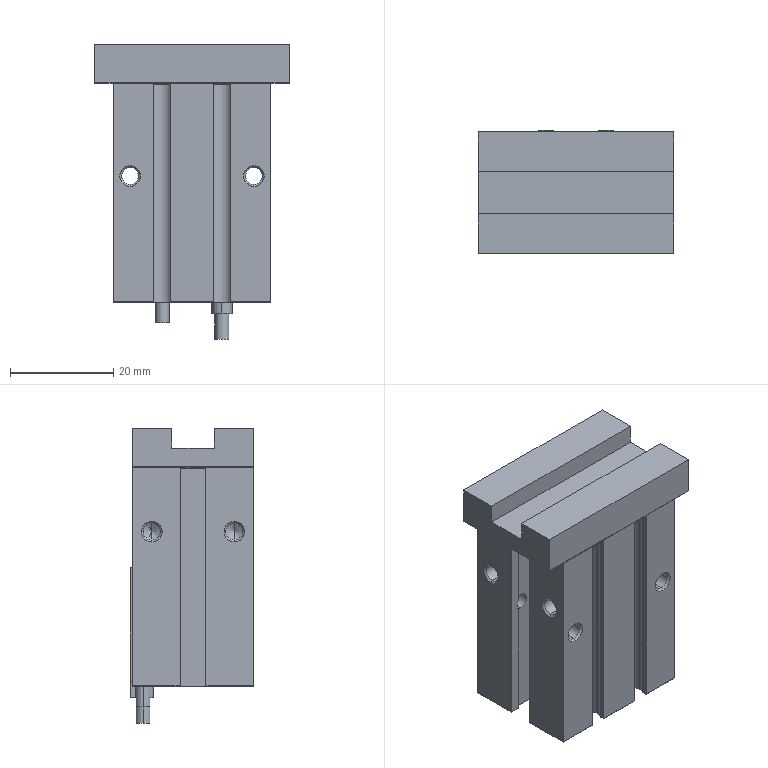Part | STEP file | MHZ2_16D | 1 solid | 159 faces | box 38 x 24 x 57.2 mm | volume 30555 mm3 | plane 85 | cylinder 46 | cone 28 | commonest cylinder face diameters 3.24 x16 4.02 x12 4 x6 2.7 x4 4.48 x4 3 x2